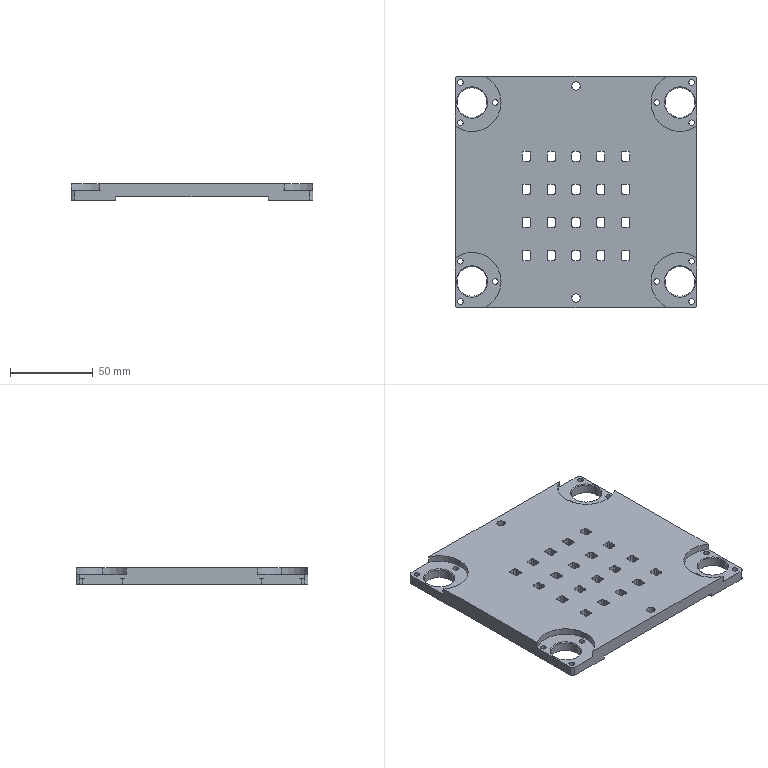Part | STEP file | FBDS-CS-026 | 1 solid | 272 faces | box 146 x 140 x 10 mm | volume 153176 mm3 | cylinder 150 | plane 110 | cone 12 | commonest cylinder face diameters 2 x80 3.4 x24 6 x24 18 x8 35 x6 4 x4